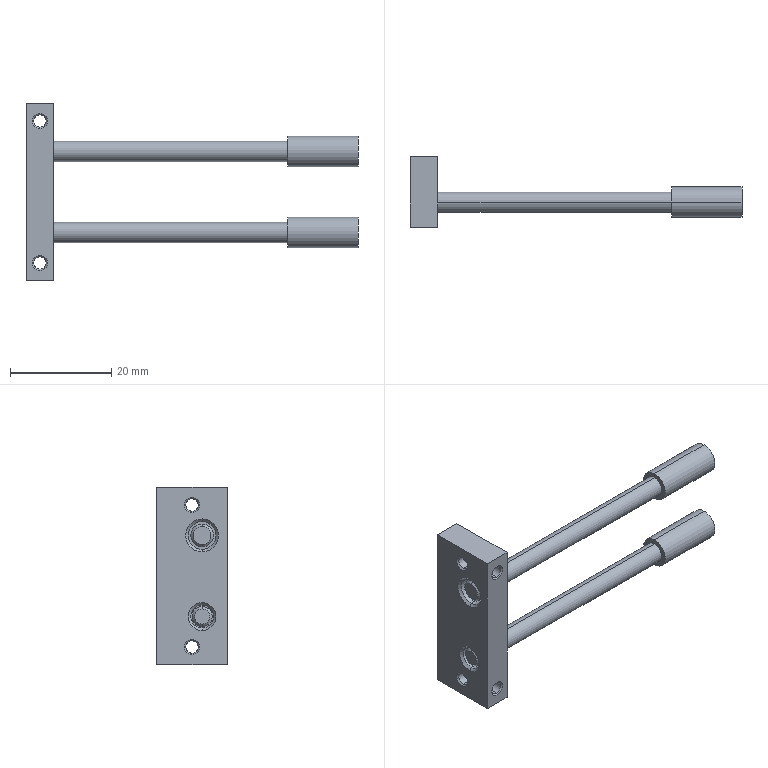Part | STEP file | _TR6-10_fr | 1 solid | 78 faces | box 65.5 x 14 x 35 mm | volume 4387 mm3 | cylinder 36 | cone 24 | plane 16 | spline 2 | commonest cylinder face diameters 2.459 x16 4 x6 4.5 x4 6 x4 3 x2 3.3 x2